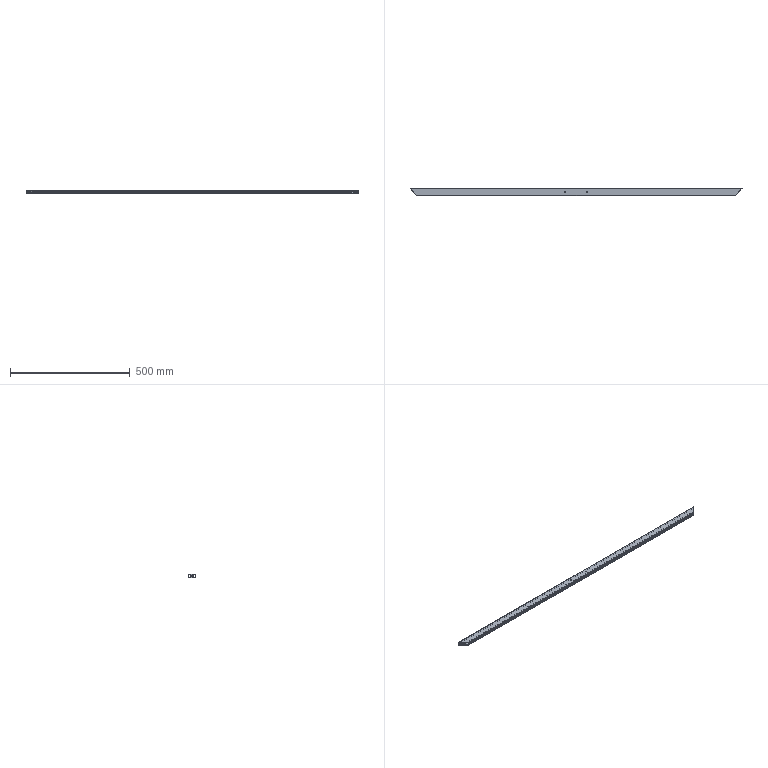Part | SolidWorks | features 3DProfileFeature 1, HoleWzd 1, ICE 1, WeldMemberFeat 1, WeldmentFeature 1 | 1 solid | 40 faces | box 1386 x 30 x 15 mm | volume 334202 mm3 | cylinder 20 | plane 20 | commonest cylinder face diameters 5 x14 3 x4 12 x2
STEP:
#1=CARTESIAN_POINT('',(-45.,-2.5,0.));
#2=VERTEX_POINT('',#1);
#3=CARTESIAN_POINT('',(-47.5,0.,2.5));
#4=VERTEX_POINT('',#3);
#5=CARTESIAN_POINT('',(-45.,-2.5,0.));
#6=CARTESIAN_POINT('',(-46.464,-2.5,1.464));
#7=CARTESIAN_POINT('',(-47.5,-1.464,2.5));
#8=CARTESIAN_POINT('',(-47.5,0.,2.5));
#9=(BOUNDED_CURVE()B_SPLINE_CURVE(3,(#5,#6,#7,#8),.UNSPECIFIED.,.F.,.F.)B_SPLINE_CURVE_WITH_KNOTS((4,4),(4.712,6.283),.UNSPECIFIED.)CURVE()GEOMETRIC_REPRESENTATION_ITEM()RATIONAL_B_SPLINE_CURVE((1.,0.8047,0.8047,1.))REPRESENTATION_ITEM(''));
#10=EDGE_CURVE('',#2,#4,#9,.T.);
#11=ORIENTED_EDGE('',*,*,#10,.T.);
#12=CARTESIAN_POINT('',(-47.5,0.,7.5));
#13=VERTEX_POINT('',#12);
#14=CARTESIAN_POINT('',(-47.5,0.,7.5));
#15=DIRECTION('',(0.,0.,1.));
#16=VECTOR('',#15,1000.);
#17=LINE('',#14,#16);
#18=EDGE_CURVE('',#4,#13,#17,.T.);
#19=ORIENTED_EDGE('',*,*,#18,.T.);
#20=CARTESIAN_POINT('',(-42.5,0.,7.5));
#21=VERTEX_POINT('',#20);
#22=CARTESIAN_POINT('',(-45.,0.,7.5));
#23=DIRECTION('',(0.,0.,1.));
#24=DIRECTION('',(1.,0.,0.));
#25=AXIS2_PLACEMENT_3D('',#22,#23,#24);
#26=CIRCLE('',#25,2.5);
#27=EDGE_CURVE('',#13,#21,#26,.T.);
#28=ORIENTED_EDGE('',*,*,#27,.T.);
#29=CARTESIAN_POINT('',(-42.5,0.,2.5));
#30=VERTEX_POINT('',#29);
#31=CARTESIAN_POINT('',(-42.5,0.,7.5));
#32=DIRECTION('',(0.,0.,1.));
#33=VECTOR('',#32,1000.);
#34=LINE('',#31,#33);
#35=EDGE_CURVE('',#30,#21,#34,.T.);
#36=ORIENTED_EDGE('',*,*,#35,.F.);
#37=CARTESIAN_POINT('',(-42.5,0.,2.5));
#38=CARTESIAN_POINT('',(-42.5,-1.464,2.5));
#39=CARTESIAN_POINT('',(-43.536,-2.5,1.464));
#40=CARTESIAN_POINT('',(-45.,-2.5,0.));
#41=(BOUNDED_CURVE()B_SPLINE_CURVE(3,(#37,#38,#39,#40),.UNSPECIFIED.,.F.,.F.)B_SPLINE_CURVE_WITH_KNOTS((4,4),(3.142,4.712),.UNSPECIFIED.)CURVE()GEOMETRIC_REPRESENTATION_ITEM()RATIONAL_B_SPLINE_CURVE((1.,0.8047,0.8047,1.))REPRESENTATION_ITEM(''));
#42=EDGE_CURVE('',#30,#2,#41,.T.);
#43=ORIENTED_EDGE('',*,*,#42,.T.);
#44=EDGE_LOOP('',(#11,#19,#28,#36,#43));
#45=FACE_OUTER_BOUND('',#44,.T.);
#46=CARTESIAN_POINT('',(-45.,0.,7.5));
#47=DIRECTION('',(0.,0.,1.));
#48=DIRECTION('',(1.,0.,0.));
#49=AXIS2_PLACEMENT_3D('',#46,#47,#48);
#50=CYLINDRICAL_SURFACE('',#49,2.5);
#51=ADVANCED_FACE('',(#45),#50,.F.);
#52=CARTESIAN_POINT('',(-47.5,0.,-7.5));
#53=VERTEX_POINT('',#52);
#54=CARTESIAN_POINT('',(-42.5,0.,-7.5));
#55=VERTEX_POINT('',#54);
#56=CARTESIAN_POINT('',(-45.,0.,-7.5));
#57=DIRECTION('',(0.,0.,1.));
#58=DIRECTION('',(1.,0.,0.));
#59=AXIS2_PLACEMENT_3D('',#56,#57,#58);
#60=CIRCLE('',#59,2.5);
#61=EDGE_CURVE('',#53,#55,#60,.T.);
#62=ORIENTED_EDGE('',*,*,#61,.F.);
#63=CARTESIAN_POINT('',(-47.5,0.,-2.5));
#64=VERTEX_POINT('',#63);
#65=CARTESIAN_POINT('',(-47.5,0.,7.5));
#66=DIRECTION('',(0.,0.,1.));
#67=VECTOR('',#66,1000.);
#68=LINE('',#65,#67);
#69=EDGE_CURVE('',#53,#64,#68,.T.);
#70=ORIENTED_EDGE('',*,*,#69,.T.);
#71=CARTESIAN_POINT('',(-47.5,0.,-2.5));
#72=CARTESIAN_POINT('',(-47.5,-1.464,-2.5));
#73=CARTESIAN_POINT('',(-46.464,-2.5,-1.464));
#74=CARTESIAN_POINT('',(-45.,-2.5,0.));
#75=(BOUNDED_CURVE()B_SPLINE_CURVE(3,(#71,#72,#73,#74),.UNSPECIFIED.,.F.,.F.)B_SPLINE_CURVE_WITH_KNOTS((4,4),(0.,1.571),.UNSPECIFIED.)CURVE()GEOMETRIC_REPRESENTATION_ITEM()RATIONAL_B_SPLINE_CURVE((1.,0.8047,0.8047,1.))REPRESENTATION_ITEM(''));
#76=EDGE_CURVE('',#64,#2,#75,.T.);
#77=ORIENTED_EDGE('',*,*,#76,.T.);
#78=CARTESIAN_POINT('',(-42.5,0.,-2.5));
#79=VERTEX_POINT('',#78);
#80=CARTESIAN_POINT('',(-45.,-2.5,0.));
#81=CARTESIAN_POINT('',(-43.536,-2.5,-1.464));
#82=CARTESIAN_POINT('',(-42.5,-1.464,-2.5));
#83=CARTESIAN_POINT('',(-42.5,0.,-2.5));
#84=(BOUNDED_CURVE()B_SPLINE_CURVE(3,(#80,#81,#82,#83),.UNSPECIFIED.,.F.,.T.)B_SPLINE_CURVE_WITH_KNOTS((4,4),(1.571,3.142),.UNSPECIFIED.)CURVE()GEOMETRIC_REPRESENTATION_ITEM()RATIONAL_B_SPLINE_CURVE((1.,0.8047,0.8047,1.))REPRESENTATION_ITEM(''));
#85=EDGE_CURVE('',#2,#79,#84,.T.);
#86=ORIENTED_EDGE('',*,*,#85,.T.);
#87=CARTESIAN_POINT('',(-42.5,0.,7.5));
#88=DIRECTION('',(0.,0.,1.));
#89=VECTOR('',#88,1000.);
#90=LINE('',#87,#89);
#91=EDGE_CURVE('',#55,#79,#90,.T.);
#92=ORIENTED_EDGE('',*,*,#91,.F.);
#93=EDGE_LOOP('',(#62,#70,#77,#86,#92));
#94=FACE_OUTER_BOUND('',#93,.T.);
#95=CARTESIAN_POINT('',(-45.,0.,7.5));
#96=DIRECTION('',(0.,0.,1.));
#97=DIRECTION('',(1.,0.,0.));
#98=AXIS2_PLACEMENT_3D('',#95,#96,#97);
#99=CYLINDRICAL_SURFACE('',#98,2.5);
#100=ADVANCED_FACE('',(#94),#99,.F.);
#101=CARTESIAN_POINT('',(45.,-2.5,0.));
#102=VERTEX_POINT('',#101);
#103=CARTESIAN_POINT('',(42.5,0.,2.5));
#104=VERTEX_POINT('',#103);
#105=CARTESIAN_POINT('',(45.,-2.5,0.));
#106=CARTESIAN_POINT('',(43.536,-2.5,1.464));
#107=CARTESIAN_POINT('',(42.5,-1.464,2.5));
#108=CARTESIAN_POINT('',(42.5,0.,2.5));
#109=(BOUNDED_CURVE()B_SPLINE_CURVE(3,(#105,#106,#107,#108),.UNSPECIFIED.,.F.,.F.)B_SPLINE_CURVE_WITH_KNOTS((4,4),(4.712,6.283),.UNSPECIFIED.)CURVE()GEOMETRIC_REPRESENTATION_ITEM()RATIONAL_B_SPLINE_CURVE((1.,0.8047,0.8047,1.))REPRESENTATION_ITEM(''));
#110=EDGE_CURVE('',#102,#104,#109,.T.);
#111=ORIENTED_EDGE('',*,*,#110,.T.);
#112=CARTESIAN_POINT('',(42.5,0.,7.5));
#113=VERTEX_POINT('',#112);
#114=CARTESIAN_POINT('',(42.5,0.,7.5));
#115=DIRECTION('',(0.,0.,1.));
#116=VECTOR('',#115,1000.);
#117=LINE('',#114,#116);
#118=EDGE_CURVE('',#104,#113,#117,.T.);
#119=ORIENTED_EDGE('',*,*,#118,.T.);
#120=CARTESIAN_POINT('',(47.5,0.,7.5));
#121=VERTEX_POINT('',#120);
#122=CARTESIAN_POINT('',(45.,0.,7.5));
#123=DIRECTION('',(0.,0.,1.));
#124=DIRECTION('',(1.,0.,0.));
#125=AXIS2_PLACEMENT_3D('',#122,#123,#124);
#126=CIRCLE('',#125,2.5);
#127=EDGE_CURVE('',#113,#121,#126,.T.);
#128=ORIENTED_EDGE('',*,*,#127,.T.);
#129=CARTESIAN_POINT('',(47.5,0.,2.5));
#130=VERTEX_POINT('',#129);
#131=CARTESIAN_POINT('',(47.5,0.,7.5));
#132=DIRECTION('',(0.,0.,1.));
#133=VECTOR('',#132,1000.);
#134=LINE('',#131,#133);
#135=EDGE_CURVE('',#130,#121,#134,.T.);
#136=ORIENTED_EDGE('',*,*,#135,.F.);
#137=CARTESIAN_POINT('',(47.5,0.,2.5));
#138=CARTESIAN_POINT('',(47.5,-1.464,2.5));
#139=CARTESIAN_POINT('',(46.464,-2.5,1.464));
#140=CARTESIAN_POINT('',(45.,-2.5,0.));
#141=(BOUNDED_CURVE()B_SPLINE_CURVE(3,(#137,#138,#139,#140),.UNSPECIFIED.,.F.,.F.)B_SPLINE_CURVE_WITH_KNOTS((4,4),(3.142,4.712),.UNSPECIFIED.)CURVE()GEOMETRIC_REPRESENTATION_ITEM()RATIONAL_B_SPLINE_CURVE((1.,0.8047,0.8047,1.))REPRESENTATION_ITEM(''));
#142=EDGE_CURVE('',#130,#102,#141,.T.);
#143=ORIENTED_EDGE('',*,*,#142,.T.);
#144=EDGE_LOOP('',(#111,#119,#128,#136,#143));
#145=FACE_OUTER_BOUND('',#144,.T.);
#146=CARTESIAN_POINT('',(45.,0.,7.5));
#147=DIRECTION('',(0.,0.,1.));
#148=DIRECTION('',(1.,0.,0.));
#149=AXIS2_PLACEMENT_3D('',#146,#147,#148);
#150=CYLINDRICAL_SURFACE('',#149,2.5);
#151=ADVANCED_FACE('',(#145),#150,.F.);
#152=CARTESIAN_POINT('',(42.5,0.,-7.5));
#153=VERTEX_POINT('',#152);
#154=CARTESIAN_POINT('',(47.5,0.,-7.5));
#155=VERTEX_POINT('',#154);
#156=CARTESIAN_POINT('',(45.,0.,-7.5));
#157=DIRECTION('',(0.,0.,1.));
#158=DIRECTION('',(1.,0.,0.));
#159=AXIS2_PLACEMENT_3D('',#156,#157,#158);
#160=CIRCLE('',#159,2.5);
#161=EDGE_CURVE('',#153,#155,#160,.T.);
#162=ORIENTED_EDGE('',*,*,#161,.F.);
#163=CARTESIAN_POINT('',(42.5,0.,-2.5));
#164=VERTEX_POINT('',#163);
#165=CARTESIAN_POINT('',(42.5,0.,7.5));
#166=DIRECTION('',(0.,0.,1.));
#167=VECTOR('',#166,1000.);
#168=LINE('',#165,#167);
#169=EDGE_CURVE('',#153,#164,#168,.T.);
#170=ORIENTED_EDGE('',*,*,#169,.T.);
#171=CARTESIAN_POINT('',(42.5,0.,-2.5));
#172=CARTESIAN_POINT('',(42.5,-1.464,-2.5));
#173=CARTESIAN_POINT('',(43.536,-2.5,-1.464));
#174=CARTESIAN_POINT('',(45.,-2.5,0.));
#175=(BOUNDED_CURVE()B_SPLINE_CURVE(3,(#171,#172,#173,#174),.UNSPECIFIED.,.F.,.T.)B_SPLINE_CURVE_WITH_KNOTS((4,4),(0.,1.571),.UNSPECIFIED.)CURVE()GEOMETRIC_REPRESENTATION_ITEM()RATIONAL_B_SPLINE_CURVE((1.,0.8047,0.8047,1.))REPRESENTATION_ITEM(''));
#176=EDGE_CURVE('',#164,#102,#175,.T.);
#177=ORIENTED_EDGE('',*,*,#176,.T.);
#178=CARTESIAN_POINT('',(47.5,0.,-2.5));
#179=VERTEX_POINT('',#178);
#180=CARTESIAN_POINT('',(45.,-2.5,0.));
#181=CARTESIAN_POINT('',(46.464,-2.5,-1.464));
#182=CARTESIAN_POINT('',(47.5,-1.464,-2.5));
#183=CARTESIAN_POINT('',(47.5,0.,-2.5));
#184=(BOUNDED_CURVE()B_SPLINE_CURVE(3,(#180,#181,#182,#183),.UNSPECIFIED.,.F.,.F.)B_SPLINE_CURVE_WITH_KNOTS((4,4),(1.571,3.142),.UNSPECIFIED.)CURVE()GEOMETRIC_REPRESENTATION_ITEM()RATIONAL_B_SPLINE_CURVE((1.,0.8047,0.8047,1.))REPRESENTATION_ITEM(''));
#185=EDGE_CURVE('',#102,#179,#184,.T.);
#186=ORIENTED_EDGE('',*,*,#185,.T.);
#187=CARTESIAN_POINT('',(47.5,0.,7.5));
#188=DIRECTION('',(0.,0.,1.));
#189=VECTOR('',#188,1000.);
#190=LINE('',#187,#189);
#191=EDGE_CURVE('',#155,#179,#190,.T.);
#192=ORIENTED_EDGE('',*,*,#191,.F.);
#193=EDGE_LOOP('',(#162,#170,#177,#186,#192));
#194=FACE_OUTER_BOUND('',#193,.T.);
#195=CARTESIAN_POINT('',(45.,0.,7.5));
#196=DIRECTION('',(0.,0.,1.));
#197=DIRECTION('',(1.,0.,0.));
#198=AXIS2_PLACEMENT_3D('',#195,#196,#197);
#199=CYLINDRICAL_SURFACE('',#198,2.5);
#200=ADVANCED_FACE('',(#194),#199,.F.);
#201=ORIENTED_EDGE('',*,*,#76,.F.);
#202=CARTESIAN_POINT('',(-678.,0.,-2.5));
#203=VERTEX_POINT('',#202);
#204=CARTESIAN_POINT('',(693.,0.,-2.5));
#205=DIRECTION('',(-1.,0.,0.));
#206=VECTOR('',#205,1000.);
#207=LINE('',#204,#206);
#208=EDGE_CURVE('',#64,#203,#207,.T.);
#209=ORIENTED_EDGE('',*,*,#208,.T.);
#210=CARTESIAN_POINT('',(-678.,0.,2.5));
#211=VERTEX_POINT('',#210);
#212=CARTESIAN_POINT('',(-678.,0.,2.5));
#213=CARTESIAN_POINT('',(-673.,-5.,2.5));
#214=CARTESIAN_POINT('',(-673.,-5.,-2.5));
#215=CARTESIAN_POINT('',(-678.,0.,-2.5));
#216=(BOUNDED_CURVE()B_SPLINE_CURVE(3,(#212,#213,#214,#215),.UNSPECIFIED.,.F.,.F.)B_SPLINE_CURVE_WITH_KNOTS((4,4),(1.571,4.712),.UNSPECIFIED.)CURVE()GEOMETRIC_REPRESENTATION_ITEM()RATIONAL_B_SPLINE_CURVE((1.,0.3333,0.3333,1.))REPRESENTATION_ITEM(''));
#217=EDGE_CURVE('',#211,#203,#216,.T.);
#218=ORIENTED_EDGE('',*,*,#217,.F.);
#219=CARTESIAN_POINT('',(693.,0.,2.5));
#220=DIRECTION('',(-1.,0.,0.));
#221=VECTOR('',#220,1000.);
#222=LINE('',#219,#221);
#223=EDGE_CURVE('',#4,#211,#222,.T.);
#224=ORIENTED_EDGE('',*,*,#223,.F.);
#225=ORIENTED_EDGE('',*,*,#10,.F.);
#226=EDGE_LOOP('',(#201,#209,#218,#224,#225));
#227=FACE_OUTER_BOUND('',#226,.T.);
#228=CARTESIAN_POINT('',(693.,0.,0.));
#229=DIRECTION('',(-1.,0.,0.));
#230=DIRECTION('',(0.,0.,1.));
#231=AXIS2_PLACEMENT_3D('',#228,#229,#230);
#232=CYLINDRICAL_SURFACE('',#231,2.5);
#233=ADVANCED_FACE('',(#227),#232,.F.);
#234=CARTESIAN_POINT('',(678.,0.,-2.5));
#235=VERTEX_POINT('',#234);
#236=CARTESIAN_POINT('',(678.,0.,2.5));
#237=VERTEX_POINT('',#236);
#238=CARTESIAN_POINT('',(678.,0.,-2.5));
#239=CARTESIAN_POINT('',(673.,-5.,-2.5));
#240=CARTESIAN_POINT('',(673.,-5.,2.5));
#241=CARTESIAN_POINT('',(678.,0.,2.5));
#242=(BOUNDED_CURVE()B_SPLINE_CURVE(3,(#238,#239,#240,#241),.UNSPECIFIED.,.F.,.F.)B_SPLINE_CURVE_WITH_KNOTS((4,4),(4.712,7.854),.UNSPECIFIED.)CURVE()GEOMETRIC_REPRESENTATION_ITEM()RATIONAL_B_SPLINE_CURVE((1.,0.3333,0.3333,1.))REPRESENTATION_ITEM(''));
#243=EDGE_CURVE('',#235,#237,#242,.T.);
#244=ORIENTED_EDGE('',*,*,#243,.F.);
#245=CARTESIAN_POINT('',(693.,0.,-2.5));
#246=DIRECTION('',(-1.,0.,0.));
#247=VECTOR('',#246,1000.);
#248=LINE('',#245,#247);
#249=EDGE_CURVE('',#235,#179,#248,.T.);
#250=ORIENTED_EDGE('',*,*,#249,.T.);
#251=ORIENTED_EDGE('',*,*,#185,.F.);
#252=ORIENTED_EDGE('',*,*,#142,.F.);
#253=CARTESIAN_POINT('',(693.,0.,2.5));
#254=DIRECTION('',(-1.,0.,0.));
#255=VECTOR('',#254,1000.);
#256=LINE('',#253,#255);
#257=EDGE_CURVE('',#237,#130,#256,.T.);
#258=ORIENTED_EDGE('',*,*,#257,.F.);
#259=EDGE_LOOP('',(#244,#250,#251,#252,#258));
#260=FACE_OUTER_BOUND('',#259,.T.);
#261=CARTESIAN_POINT('',(693.,0.,0.));
#262=DIRECTION('',(-1.,0.,0.));
#263=DIRECTION('',(0.,0.,1.));
#264=AXIS2_PLACEMENT_3D('',#261,#262,#263);
#265=CYLINDRICAL_SURFACE('',#264,2.5);
#266=ADVANCED_FACE('',(#260),#265,.F.);
#267=ORIENTED_EDGE('',*,*,#176,.F.);
#268=CARTESIAN_POINT('',(693.,0.,-2.5));
#269=DIRECTION('',(-1.,0.,0.));
#270=VECTOR('',#269,1000.);
#271=LINE('',#268,#270);
#272=EDGE_CURVE('',#164,#79,#271,.T.);
#273=ORIENTED_EDGE('',*,*,#272,.T.);
#274=ORIENTED_EDGE('',*,*,#85,.F.);
#275=ORIENTED_EDGE('',*,*,#42,.F.);
#276=CARTESIAN_POINT('',(693.,0.,2.5));
#277=DIRECTION('',(-1.,0.,0.));
#278=VECTOR('',#277,1000.);
#279=LINE('',#276,#278);
#280=EDGE_CURVE('',#104,#30,#279,.T.);
#281=ORIENTED_EDGE('',*,*,#280,.F.);
#282=ORIENTED_EDGE('',*,*,#110,.F.);
#283=EDGE_LOOP('',(#267,#273,#274,#275,#281,#282));
#284=FACE_OUTER_BOUND('',#283,.T.);
#285=CARTESIAN_POINT('',(693.,0.,0.));
#286=DIRECTION('',(-1.,0.,0.));
#287=DIRECTION('',(0.,0.,1.));
#288=AXIS2_PLACEMENT_3D('',#285,#286,#287);
#289=CYLINDRICAL_SURFACE('',#288,2.5);
#290=ADVANCED_FACE('',(#284),#289,.F.);
#291=ORIENTED_EDGE('',*,*,#272,.F.);
#292=CARTESIAN_POINT('',(45.,2.5,0.));
#293=VERTEX_POINT('',#292);
#294=CARTESIAN_POINT('',(45.,2.5,0.));
#295=CARTESIAN_POINT('',(43.536,2.5,-1.464));
#296=CARTESIAN_POINT('',(42.5,1.464,-2.5));
#297=CARTESIAN_POINT('',(42.5,0.,-2.5));
#298=(BOUNDED_CURVE()B_SPLINE_CURVE(3,(#294,#295,#296,#297),.UNSPECIFIED.,.F.,.F.)B_SPLINE_CURVE_WITH_KNOTS((4,4),(4.712,6.283),.UNSPECIFIED.)CURVE()GEOMETRIC_REPRESENTATION_ITEM()RATIONAL_B_SPLINE_CURVE((1.,0.8047,0.8047,1.))REPRESENTATION_ITEM(''));
#299=EDGE_CURVE('',#293,#164,#298,.T.);
#300=ORIENTED_EDGE('',*,*,#299,.F.);
#301=CARTESIAN_POINT('',(42.5,0.,2.5));
#302=CARTESIAN_POINT('',(42.5,1.464,2.5));
#303=CARTESIAN_POINT('',(43.536,2.5,1.464));
#304=CARTESIAN_POINT('',(45.,2.5,0.));
#305=(BOUNDED_CURVE()B_SPLINE_CURVE(3,(#301,#302,#303,#304),.UNSPECIFIED.,.F.,.F.)B_SPLINE_CURVE_WITH_KNOTS((4,4),(0.,1.571),.UNSPECIFIED.)CURVE()GEOMETRIC_REPRESENTATION_ITEM()RATIONAL_B_SPLINE_CURVE((1.,0.8047,0.8047,1.))REPRESENTATION_ITEM(''));
#306=EDGE_CURVE('',#104,#293,#305,.T.);
#307=ORIENTED_EDGE('',*,*,#306,.F.);
#308=ORIENTED_EDGE('',*,*,#280,.T.);
#309=CARTESIAN_POINT('',(-45.,2.5,0.));
#310=VERTEX_POINT('',#309);
#311=CARTESIAN_POINT('',(-45.,2.5,0.));
#312=CARTESIAN_POINT('',(-43.536,2.5,1.464));
#313=CARTESIAN_POINT('',(-42.5,1.464,2.5));
#314=CARTESIAN_POINT('',(-42.5,0.,2.5));
#315=(BOUNDED_CURVE()B_SPLINE_CURVE(3,(#311,#312,#313,#314),.UNSPECIFIED.,.F.,.F.)B_SPLINE_CURVE_WITH_KNOTS((4,4),(1.571,3.142),.UNSPECIFIED.)CURVE()GEOMETRIC_REPRESENTATION_ITEM()RATIONAL_B_SPLINE_CURVE((1.,0.8047,0.8047,1.))REPRESENTATION_ITEM(''));
#316=EDGE_CURVE('',#310,#30,#315,.T.);
#317=ORIENTED_EDGE('',*,*,#316,.F.);
#318=CARTESIAN_POINT('',(-42.5,0.,-2.5));
#319=CARTESIAN_POINT('',(-42.5,1.464,-2.5));
#320=CARTESIAN_POINT('',(-43.536,2.5,-1.464));
#321=CARTESIAN_POINT('',(-45.,2.5,0.));
#322=(BOUNDED_CURVE()B_SPLINE_CURVE(3,(#318,#319,#320,#321),.UNSPECIFIED.,.F.,.F.)B_SPLINE_CURVE_WITH_KNOTS((4,4),(3.142,4.712),.UNSPECIFIED.)CURVE()GEOMETRIC_REPRESENTATION_ITEM()RATIONAL_B_SPLINE_CURVE((1.,0.8047,0.8047,1.))REPRESENTATION_ITEM(''));
#323=EDGE_CURVE('',#79,#310,#322,.T.);
#324=ORIENTED_EDGE('',*,*,#323,.F.);
#325=EDGE_LOOP('',(#291,#300,#307,#308,#317,#324));
#326=FACE_OUTER_BOUND('',#325,.T.);
#327=CARTESIAN_POINT('',(693.,0.,0.));
#328=DIRECTION('',(-1.,0.,0.));
#329=DIRECTION('',(0.,0.,1.));
#330=AXIS2_PLACEMENT_3D('',#327,#328,#329);
#331=CYLINDRICAL_SURFACE('',#330,2.5);
#332=ADVANCED_FACE('',(#326),#331,.F.);
#333=ORIENTED_EDGE('',*,*,#249,.F.);
#334=CARTESIAN_POINT('',(678.,0.,2.5));
#335=CARTESIAN_POINT('',(683.,5.,2.5));
#336=CARTESIAN_POINT('',(683.,5.,-2.5));
#337=CARTESIAN_POINT('',(678.,0.,-2.5));
#338=(BOUNDED_CURVE()B_SPLINE_CURVE(3,(#334,#335,#336,#337),.UNSPECIFIED.,.F.,.T.)B_SPLINE_CURVE_WITH_KNOTS((4,4),(1.571,4.712),.UNSPECIFIED.)CURVE()GEOMETRIC_REPRESENTATION_ITEM()RATIONAL_B_SPLINE_CURVE((1.,0.3333,0.3333,1.))REPRESENTATION_ITEM(''));
#339=EDGE_CURVE('',#237,#235,#338,.T.);
#340=ORIENTED_EDGE('',*,*,#339,.F.);
#341=ORIENTED_EDGE('',*,*,#257,.T.);
#342=CARTESIAN_POINT('',(45.,2.5,0.));
#343=CARTESIAN_POINT('',(46.464,2.5,1.464));
#344=CARTESIAN_POINT('',(47.5,1.464,2.5));
#345=CARTESIAN_POINT('',(47.5,0.,2.5));
#346=(BOUNDED_CURVE()B_SPLINE_CURVE(3,(#342,#343,#344,#345),.UNSPECIFIED.,.F.,.F.)B_SPLINE_CURVE_WITH_KNOTS((4,4),(1.571,3.142),.UNSPECIFIED.)CURVE()GEOMETRIC_REPRESENTATION_ITEM()RATIONAL_B_SPLINE_CURVE((1.,0.8047,0.8047,1.))REPRESENTATION_ITEM(''));
#347=EDGE_CURVE('',#293,#130,#346,.T.);
#348=ORIENTED_EDGE('',*,*,#347,.F.);
#349=CARTESIAN_POINT('',(47.5,0.,-2.5));
#350=CARTESIAN_POINT('',(47.5,1.464,-2.5));
#351=CARTESIAN_POINT('',(46.464,2.5,-1.464));
#352=CARTESIAN_POINT('',(45.,2.5,0.));
#353=(BOUNDED_CURVE()B_SPLINE_CURVE(3,(#349,#350,#351,#352),.UNSPECIFIED.,.F.,.F.)B_SPLINE_CURVE_WITH_KNOTS((4,4),(3.142,4.712),.UNSPECIFIED.)CURVE()GEOMETRIC_REPRESENTATION_ITEM()RATIONAL_B_SPLINE_CURVE((1.,0.8047,0.8047,1.))REPRESENTATION_ITEM(''));
#354=EDGE_CURVE('',#179,#293,#353,.T.);
#355=ORIENTED_EDGE('',*,*,#354,.F.);
#356=EDGE_LOOP('',(#333,#340,#341,#348,#355));
#357=FACE_OUTER_BOUND('',#356,.T.);
#358=CARTESIAN_POINT('',(693.,0.,0.));
#359=DIRECTION('',(-1.,0.,0.));
#360=DIRECTION('',(0.,0.,1.));
#361=AXIS2_PLACEMENT_3D('',#358,#359,#360);
#362=CYLINDRICAL_SURFACE('',#361,2.5);
#363=ADVANCED_FACE('',(#357),#362,.F.);
#364=CARTESIAN_POINT('',(693.,15.,3.25));
#365=VERTEX_POINT('',#364);
#366=CARTESIAN_POINT('',(-693.,15.,3.25));
#367=VERTEX_POINT('',#366);
#368=CARTESIAN_POINT('',(693.,15.,3.25));
#369=DIRECTION('',(-1.,0.,0.));
#370=VECTOR('',#369,1000.);
#371=LINE('',#368,#370);
#372=EDGE_CURVE('',#365,#367,#371,.T.);
#373=ORIENTED_EDGE('',*,*,#372,.F.);
#374=CARTESIAN_POINT('',(690.7,12.7,3.25));
#375=VERTEX_POINT('',#374);
#376=CARTESIAN_POINT('',(693.,15.,3.25));
#377=DIRECTION('',(-0.7071,-0.7071,0.));
#378=VECTOR('',#377,1000.);
#379=LINE('',#376,#378);
#380=EDGE_CURVE('',#365,#375,#379,.T.);
#381=ORIENTED_EDGE('',*,*,#380,.T.);
#382=CARTESIAN_POINT('',(-690.7,12.7,3.25));
#383=VERTEX_POINT('',#382);
#384=CARTESIAN_POINT('',(693.,12.7,3.25));
#385=DIRECTION('',(-1.,0.,0.));
#386=VECTOR('',#385,1000.);
#387=LINE('',#384,#386);
#388=EDGE_CURVE('',#375,#383,#387,.T.);
#389=ORIENTED_EDGE('',*,*,#388,.T.);
#390=CARTESIAN_POINT('',(0.,-678.,3.25));
#391=DIRECTION('',(-0.7071,0.7071,0.));
#392=VECTOR('',#391,1000.);
#393=LINE('',#390,#392);
#394=EDGE_CURVE('',#383,#367,#393,.T.);
#395=ORIENTED_EDGE('',*,*,#394,.T.);
#396=EDGE_LOOP('',(#373,#381,#389,#395));
#397=FACE_OUTER_BOUND('',#396,.T.);
#398=CARTESIAN_POINT('',(693.,15.,3.25));
#399=DIRECTION('',(0.,0.,1.));
#400=DIRECTION('',(0.,-1.,0.));
#401=AXIS2_PLACEMENT_3D('',#398,#399,#400);
#402=PLANE('',#401);
#403=ADVANCED_FACE('',(#397),#402,.F.);
#404=CARTESIAN_POINT('',(-693.,15.,6.));
#405=VERTEX_POINT('',#404);
#406=CARTESIAN_POINT('',(-693.,15.,6.));
#407=DIRECTION('',(0.,0.,1.));
#408=VECTOR('',#407,1000.);
#409=LINE('',#406,#408);
#410=EDGE_CURVE('',#367,#405,#409,.T.);
#411=ORIENTED_EDGE('',*,*,#410,.T.);
#412=CARTESIAN_POINT('',(693.,15.,6.));
#413=VERTEX_POINT('',#412);
#414=CARTESIAN_POINT('',(693.,15.,6.));
#415=DIRECTION('',(-1.,0.,0.));
#416=VECTOR('',#415,1000.);
#417=LINE('',#414,#416);
#418=EDGE_CURVE('',#413,#405,#417,.T.);
#419=ORIENTED_EDGE('',*,*,#418,.F.);
#420=CARTESIAN_POINT('',(693.,15.,6.));
#421=DIRECTION('',(0.,0.,1.));
#422=VECTOR('',#421,1000.);
#423=LINE('',#420,#422);
#424=EDGE_CURVE('',#365,#413,#423,.T.);
#425=ORIENTED_EDGE('',*,*,#424,.F.);
#426=ORIENTED_EDGE('',*,*,#372,.T.);
#427=EDGE_LOOP('',(#411,#419,#425,#426));
#428=FACE_OUTER_BOUND('',#427,.T.);
#429=CARTESIAN_POINT('',(693.,15.,6.));
#430=DIRECTION('',(0.,-1.,0.));
#431=DIRECTION('',(0.,0.,-1.));
#432=AXIS2_PLACEMENT_3D('',#429,#430,#431);
#433=PLANE('',#432);
#434=ADVANCED_FACE('',(#428),#433,.F.);
#435=CARTESIAN_POINT('',(691.5,13.5,7.5));
#436=VERTEX_POINT('',#435);
#437=CARTESIAN_POINT('',(-691.5,13.5,7.5));
#438=VERTEX_POINT('',#437);
#439=CARTESIAN_POINT('',(693.,13.5,7.5));
#440=DIRECTION('',(-1.,0.,0.));
#441=VECTOR('',#440,1000.);
#442=LINE('',#439,#441);
#443=EDGE_CURVE('',#436,#438,#442,.T.);
#444=ORIENTED_EDGE('',*,*,#443,.F.);
#445=CARTESIAN_POINT('',(691.5,13.5,7.5));
#446=CARTESIAN_POINT('',(692.379,14.379,7.5));
#447=CARTESIAN_POINT('',(693.,15.,6.879));
#448=CARTESIAN_POINT('',(693.,15.,6.));
#449=(BOUNDED_CURVE()B_SPLINE_CURVE(3,(#445,#446,#447,#448),.UNSPECIFIED.,.F.,.F.)B_SPLINE_CURVE_WITH_KNOTS((4,4),(1.571,3.142),.UNSPECIFIED.)CURVE()GEOMETRIC_REPRESENTATION_ITEM()RATIONAL_B_SPLINE_CURVE((1.,0.8047,0.8047,1.))REPRESENTATION_ITEM(''));
#450=EDGE_CURVE('',#436,#413,#449,.T.);
#451=ORIENTED_EDGE('',*,*,#450,.T.);
#452=ORIENTED_EDGE('',*,*,#418,.T.);
#453=CARTESIAN_POINT('',(-693.,15.,6.));
#454=CARTESIAN_POINT('',(-693.,15.,6.879));
#455=CARTESIAN_POINT('',(-692.379,14.379,7.5));
#456=CARTESIAN_POINT('',(-691.5,13.5,7.5));
#457=(BOUNDED_CURVE()B_SPLINE_CURVE(3,(#453,#454,#455,#456),.UNSPECIFIED.,.F.,.F.)B_SPLINE_CURVE_WITH_KNOTS((4,4),(0.,1.571),.UNSPECIFIED.)CURVE()GEOMETRIC_REPRESENTATION_ITEM()RATIONAL_B_SPLINE_CURVE((1.,0.8047,0.8047,1.))REPRESENTATION_ITEM(''));
#458=EDGE_CURVE('',#405,#438,#457,.T.);
#459=ORIENTED_EDGE('',*,*,#458,.T.);
#460=EDGE_LOOP('',(#444,#451,#452,#459));
#461=FACE_OUTER_BOUND('',#460,.T.);
#462=CARTESIAN_POINT('',(693.,13.5,6.));
#463=DIRECTION('',(-1.,0.,0.));
#464=DIRECTION('',(0.,0.,1.));
#465=AXIS2_PLACEMENT_3D('',#462,#463,#464);
#466=CYLINDRICAL_SURFACE('',#465,1.5);
#467=ADVANCED_FACE('',(#461),#466,.T.);
#468=CARTESIAN_POINT('',(-45.,0.,7.5));
#469=DIRECTION('',(0.,0.,1.));
#470=DIRECTION('',(1.,0.,0.));
#471=AXIS2_PLACEMENT_3D('',#468,#469,#470);
#472=CIRCLE('',#471,2.5);
#473=EDGE_CURVE('',#21,#13,#472,.T.);
#474=ORIENTED_EDGE('',*,*,#473,.F.);
#475=ORIENTED_EDGE('',*,*,#27,.F.);
#476=EDGE_LOOP('',(#474,#475));
#477=FACE_BOUND('',#476,.T.);
#478=CARTESIAN_POINT('',(45.,0.,7.5));
#479=DIRECTION('',(0.,0.,1.));
#480=DIRECTION('',(1.,0.,0.));
#481=AXIS2_PLACEMENT_3D('',#478,#479,#480);
#482=CIRCLE('',#481,2.5);
#483=EDGE_CURVE('',#121,#113,#482,.T.);
#484=ORIENTED_EDGE('',*,*,#483,.F.);
#485=ORIENTED_EDGE('',*,*,#127,.F.);
#486=EDGE_LOOP('',(#484,#485));
#487=FACE_BOUND('',#486,.T.);
#488=CARTESIAN_POINT('',(664.5,-13.5,7.5));
#489=VERTEX_POINT('',#488);
#490=CARTESIAN_POINT('',(-664.5,-13.5,7.5));
#491=VERTEX_POINT('',#490);
#492=CARTESIAN_POINT('',(693.,-13.5,7.5));
#493=DIRECTION('',(-1.,0.,0.));
#494=VECTOR('',#493,1000.);
#495=LINE('',#492,#494);
#496=EDGE_CURVE('',#489,#491,#495,.T.);
#497=ORIENTED_EDGE('',*,*,#496,.F.);
#498=CARTESIAN_POINT('',(693.,15.,7.5));
#499=DIRECTION('',(-0.7071,-0.7071,0.));
#500=VECTOR('',#499,1000.);
#501=LINE('',#498,#500);
#502=EDGE_CURVE('',#436,#489,#501,.T.);
#503=ORIENTED_EDGE('',*,*,#502,.F.);
#504=ORIENTED_EDGE('',*,*,#443,.T.);
#505=CARTESIAN_POINT('',(-693.,15.,7.5));
#506=DIRECTION('',(-0.7071,0.7071,0.));
#507=VECTOR('',#506,1000.);
#508=LINE('',#505,#507);
#509=EDGE_CURVE('',#491,#438,#508,.T.);
#510=ORIENTED_EDGE('',*,*,#509,.F.);
#511=EDGE_LOOP('',(#497,#503,#504,#510));
#512=FACE_OUTER_BOUND('',#511,.T.);
#513=CARTESIAN_POINT('',(693.,-13.5,7.5));
#514=DIRECTION('',(0.,0.,-1.));
#515=DIRECTION('',(-1.,0.,0.));
#516=AXIS2_PLACEMENT_3D('',#513,#514,#515);
#517=PLANE('',#516);
#518=ADVANCED_FACE('',(#477,#487,#512),#517,.F.);
#519=CARTESIAN_POINT('',(663.,-15.,6.));
#520=VERTEX_POINT('',#519);
#521=CARTESIAN_POINT('',(-663.,-15.,6.));
#522=VERTEX_POINT('',#521);
#523=CARTESIAN_POINT('',(693.,-15.,6.));
#524=DIRECTION('',(-1.,0.,0.));
#525=VECTOR('',#524,1000.);
#526=LINE('',#523,#525);
#527=EDGE_CURVE('',#520,#522,#526,.T.);
#528=ORIENTED_EDGE('',*,*,#527,.F.);
#529=CARTESIAN_POINT('',(663.,-15.,6.));
#530=CARTESIAN_POINT('',(663.,-15.,6.879));
#531=CARTESIAN_POINT('',(663.621,-14.379,7.5));
#532=CARTESIAN_POINT('',(664.5,-13.5,7.5));
#533=(BOUNDED_CURVE()B_SPLINE_CURVE(3,(#529,#530,#531,#532),.UNSPECIFIED.,.F.,.F.)B_SPLINE_CURVE_WITH_KNOTS((4,4),(0.,1.571),.UNSPECIFIED.)CURVE()GEOMETRIC_REPRESENTATION_ITEM()RATIONAL_B_SPLINE_CURVE((1.,0.8047,0.8047,1.))REPRESENTATION_ITEM(''));
#534=EDGE_CURVE('',#520,#489,#533,.T.);
#535=ORIENTED_EDGE('',*,*,#534,.T.);
#536=ORIENTED_EDGE('',*,*,#496,.T.);
#537=CARTESIAN_POINT('',(-664.5,-13.5,7.5));
#538=CARTESIAN_POINT('',(-663.621,-14.379,7.5));
#539=CARTESIAN_POINT('',(-663.,-15.,6.879));
#540=CARTESIAN_POINT('',(-663.,-15.,6.));
#541=(BOUNDED_CURVE()B_SPLINE_CURVE(3,(#537,#538,#539,#540),.UNSPECIFIED.,.F.,.F.)B_SPLINE_CURVE_WITH_KNOTS((4,4),(1.571,3.142),.UNSPECIFIED.)CURVE()GEOMETRIC_REPRESENTATION_ITEM()RATIONAL_B_SPLINE_CURVE((1.,0.8047,0.8047,1.))REPRESENTATION_ITEM(''));
#542=EDGE_CURVE('',#491,#522,#541,.T.);
#543=ORIENTED_EDGE('',*,*,#542,.T.);
#544=EDGE_LOOP('',(#528,#535,#536,#543));
#545=FACE_OUTER_BOUND('',#544,.T.);
#546=CARTESIAN_POINT('',(693.,-13.5,6.));
#547=DIRECTION('',(-1.,0.,0.));
#548=DIRECTION('',(0.,0.,1.));
#549=AXIS2_PLACEMENT_3D('',#546,#547,#548);
#550=CYLINDRICAL_SURFACE('',#549,1.5);
#551=ADVANCED_FACE('',(#545),#550,.T.);
#552=CARTESIAN_POINT('',(663.,-15.,3.25));
#553=VERTEX_POINT('',#552);
#554=CARTESIAN_POINT('',(-663.,-15.,3.25));
#555=VERTEX_POINT('',#554);
#556=CARTESIAN_POINT('',(693.,-15.,3.25));
#557=DIRECTION('',(-1.,0.,0.));
#558=VECTOR('',#557,1000.);
#559=LINE('',#556,#558);
#560=EDGE_CURVE('',#553,#555,#559,.T.);
#561=ORIENTED_EDGE('',*,*,#560,.F.);
#562=CARTESIAN_POINT('',(663.,-15.,-7.5));
#563=DIRECTION('',(0.,0.,1.));
#564=VECTOR('',#563,1000.);
#565=LINE('',#562,#564);
#566=EDGE_CURVE('',#553,#520,#565,.T.);
#567=ORIENTED_EDGE('',*,*,#566,.T.);
#568=ORIENTED_EDGE('',*,*,#527,.T.);
#569=CARTESIAN_POINT('',(-663.,-15.,-7.5));
#570=DIRECTION('',(0.,0.,1.));
#571=VECTOR('',#570,1000.);
#572=LINE('',#569,#571);
#573=EDGE_CURVE('',#555,#522,#572,.T.);
#574=ORIENTED_EDGE('',*,*,#573,.F.);
#575=EDGE_LOOP('',(#561,#567,#568,#574));
#576=FACE_OUTER_BOUND('',#575,.T.);
#577=CARTESIAN_POINT('',(693.,-15.,6.));
#578=DIRECTION('',(0.,1.,0.));
#579=DIRECTION('',(0.,0.,1.));
#580=AXIS2_PLACEMENT_3D('',#577,#578,#579);
#581=PLANE('',#580);
#582=ADVANCED_FACE('',(#576),#581,.F.);
#583=CARTESIAN_POINT('',(665.3,-12.7,3.25));
#584=VERTEX_POINT('',#583);
#585=CARTESIAN_POINT('',(-665.3,-12.7,3.25));
#586=VERTEX_POINT('',#585);
#587=CARTESIAN_POINT('',(693.,-12.7,3.25));
#588=DIRECTION('',(-1.,0.,0.));
#589=VECTOR('',#588,1000.);
#590=LINE('',#587,#589);
#591=EDGE_CURVE('',#584,#586,#590,.T.);
#592=ORIENTED_EDGE('',*,*,#591,.F.);
#593=CARTESIAN_POINT('',(678.,0.,3.25));
#594=DIRECTION('',(-0.7071,-0.7071,0.));
#595=VECTOR('',#594,1000.);
#596=LINE('',#593,#595);
#597=EDGE_CURVE('',#584,#553,#596,.T.);
#598=ORIENTED_EDGE('',*,*,#597,.T.);
#599=ORIENTED_EDGE('',*,*,#560,.T.);
#600=CARTESIAN_POINT('',(15.,-693.,3.25));
#601=DIRECTION('',(-0.7071,0.7071,0.));
#602=VECTOR('',#601,1000.);
#603=LINE('',#600,#602);
#604=EDGE_CURVE('',#555,#586,#603,.T.);
#605=ORIENTED_EDGE('',*,*,#604,.T.);
#606=EDGE_LOOP('',(#592,#598,#599,#605));
#607=FACE_OUTER_BOUND('',#606,.T.);
#608=CARTESIAN_POINT('',(693.,-15.,3.25));
#609=DIRECTION('',(0.,0.,1.));
#610=DIRECTION('',(0.,-1.,0.));
#611=AXIS2_PLACEMENT_3D('',#608,#609,#610);
#612=PLANE('',#611);
#613=ADVANCED_FACE('',(#607),#612,.F.);
#614=CARTESIAN_POINT('',(665.3,-12.7,5.));
#615=VERTEX_POINT('',#614);
#616=CARTESIAN_POINT('',(-665.3,-12.7,5.));
#617=VERTEX_POINT('',#616);
#618=CARTESIAN_POINT('',(693.,-12.7,5.));
#619=DIRECTION('',(-1.,0.,0.));
#620=VECTOR('',#619,1000.);
#621=LINE('',#618,#620);
#622=EDGE_CURVE('',#615,#617,#621,.T.);
#623=ORIENTED_EDGE('',*,*,#622,.F.);
#624=CARTESIAN_POINT('',(665.3,-12.7,3.25));
#625=DIRECTION('',(0.,0.,-1.));
#626=VECTOR('',#625,1000.);
#627=LINE('',#624,#626);
#628=EDGE_CURVE('',#615,#584,#627,.T.);
#629=ORIENTED_EDGE('',*,*,#628,.T.);
#630=ORIENTED_EDGE('',*,*,#591,.T.);
#631=CARTESIAN_POINT('',(-665.3,-12.7,3.25));
#632=DIRECTION('',(0.,0.,1.));
#633=VECTOR('',#632,1000.);
#634=LINE('',#631,#633);
#635=EDGE_CURVE('',#586,#617,#634,.T.);
#636=ORIENTED_EDGE('',*,*,#635,.T.);
#637=EDGE_LOOP('',(#623,#629,#630,#636));
#638=FACE_OUTER_BOUND('',#637,.T.);
#639=CARTESIAN_POINT('',(693.,-12.7,3.25));
#640=DIRECTION('',(0.,-1.,0.));
#641=DIRECTION('',(0.,0.,-1.));
#642=AXIS2_PLACEMENT_3D('',#639,#640,#641);
#643=PLANE('',#642);
#644=ADVANCED_FACE('',(#638),#643,.F.);
#645=CARTESIAN_POINT('',(671.,-7.,5.));
#646=VERTEX_POINT('',#645);
#647=CARTESIAN_POINT('',(-671.,-7.,5.));
#648=VERTEX_POINT('',#647);
#649=CARTESIAN_POINT('',(693.,-7.,5.));
#650=DIRECTION('',(-1.,0.,0.));
#651=VECTOR('',#650,1000.);
#652=LINE('',#649,#651);
#653=EDGE_CURVE('',#646,#648,#652,.T.);
#654=ORIENTED_EDGE('',*,*,#653,.F.);
#655=CARTESIAN_POINT('',(679.15,1.15,5.));
#656=DIRECTION('',(-0.7071,-0.7071,0.));
#657=VECTOR('',#656,1000.);
#658=LINE('',#655,#657);
#659=EDGE_CURVE('',#646,#615,#658,.T.);
#660=ORIENTED_EDGE('',*,*,#659,.T.);
#661=ORIENTED_EDGE('',*,*,#622,.T.);
#662=CARTESIAN_POINT('',(13.85,-691.85,5.));
#663=DIRECTION('',(-0.7071,0.7071,0.));
#664=VECTOR('',#663,1000.);
#665=LINE('',#662,#664);
#666=EDGE_CURVE('',#617,#648,#665,.T.);
#667=ORIENTED_EDGE('',*,*,#666,.T.);
#668=EDGE_LOOP('',(#654,#660,#661,#667));
#669=FACE_OUTER_BOUND('',#668,.T.);
#670=CARTESIAN_POINT('',(693.,-12.7,5.));
#671=DIRECTION('',(0.,0.,1.));
#672=DIRECTION('',(0.,-1.,0.));
#673=AXIS2_PLACEMENT_3D('',#670,#671,#672);
#674=PLANE('',#673);
#675=ADVANCED_FACE('',(#669),#674,.F.);
#676=CARTESIAN_POINT('',(671.,-7.,-5.));
#677=VERTEX_POINT('',#676);
#678=CARTESIAN_POINT('',(-671.,-7.,-5.));
#679=VERTEX_POINT('',#678);
#680=CARTESIAN_POINT('',(693.,-7.,-5.));
#681=DIRECTION('',(-1.,0.,0.));
#682=VECTOR('',#681,1000.);
#683=LINE('',#680,#682);
#684=EDGE_CURVE('',#677,#679,#683,.T.);
#685=ORIENTED_EDGE('',*,*,#684,.F.);
#686=CARTESIAN_POINT('',(671.,-7.,-5.));
#687=CARTESIAN_POINT('',(674.958,-3.042,-2.375));
#688=CARTESIAN_POINT('',(674.958,-3.042,2.375));
#689=CARTESIAN_POINT('',(671.,-7.,5.));
#690=(BOUNDED_CURVE()B_SPLINE_CURVE(3,(#686,#687,#688,#689),.UNSPECIFIED.,.F.,.F.)B_SPLINE_CURVE_WITH_KNOTS((4,4),(2.156,4.127),.UNSPECIFIED.)CURVE()GEOMETRIC_REPRESENTATION_ITEM()RATIONAL_B_SPLINE_CURVE((1.,0.7018,0.7018,1.))REPRESENTATION_ITEM(''));
#691=EDGE_CURVE('',#677,#646,#690,.T.);
#692=ORIENTED_EDGE('',*,*,#691,.T.);
#693=ORIENTED_EDGE('',*,*,#653,.T.);
#694=CARTESIAN_POINT('',(-671.,-7.,5.));
#695=CARTESIAN_POINT('',(-674.958,-3.042,2.375));
#696=CARTESIAN_POINT('',(-674.958,-3.042,-2.375));
#697=CARTESIAN_POINT('',(-671.,-7.,-5.));
#698=(BOUNDED_CURVE()B_SPLINE_CURVE(3,(#694,#695,#696,#697),.UNSPECIFIED.,.F.,.F.)B_SPLINE_CURVE_WITH_KNOTS((4,4),(5.298,7.268),.UNSPECIFIED.)CURVE()GEOMETRIC_REPRESENTATION_ITEM()RATIONAL_B_SPLINE_CURVE((1.,0.7018,0.7018,1.))REPRESENTATION_ITEM(''));
#699=EDGE_CURVE('',#648,#679,#698,.T.);
#700=ORIENTED_EDGE('',*,*,#699,.T.);
#701=EDGE_LOOP('',(#685,#692,#693,#700));
#702=FACE_OUTER_BOUND('',#701,.T.);
#703=CARTESIAN_POINT('',(693.,-10.317,0.));
#704=DIRECTION('',(-1.,0.,0.));
#705=DIRECTION('',(0.,0.,1.));
#706=AXIS2_PLACEMENT_3D('',#703,#704,#705);
#707=CYLINDRICAL_SURFACE('',#706,6.);
#708=ADVANCED_FACE('',(#702),#707,.F.);
#709=CARTESIAN_POINT('',(665.3,-12.7,-5.));
#710=VERTEX_POINT('',#709);
#711=CARTESIAN_POINT('',(-665.3,-12.7,-5.));
#712=VERTEX_POINT('',#711);
#713=CARTESIAN_POINT('',(693.,-12.7,-5.));
#714=DIRECTION('',(-1.,0.,0.));
#715=VECTOR('',#714,1000.);
#716=LINE('',#713,#715);
#717=EDGE_CURVE('',#710,#712,#716,.T.);
#718=ORIENTED_EDGE('',*,*,#717,.F.);
#719=CARTESIAN_POINT('',(679.15,1.15,-5.));
#720=DIRECTION('',(0.7071,0.7071,0.));
#721=VECTOR('',#720,1000.);
#722=LINE('',#719,#721);
#723=EDGE_CURVE('',#710,#677,#722,.T.);
#724=ORIENTED_EDGE('',*,*,#723,.T.);
#725=ORIENTED_EDGE('',*,*,#684,.T.);
#726=CARTESIAN_POINT('',(13.85,-691.85,-5.));
#727=DIRECTION('',(0.7071,-0.7071,0.));
#728=VECTOR('',#727,1000.);
#729=LINE('',#726,#728);
#730=EDGE_CURVE('',#679,#712,#729,.T.);
#731=ORIENTED_EDGE('',*,*,#730,.T.);
#732=EDGE_LOOP('',(#718,#724,#725,#731));
#733=FACE_OUTER_BOUND('',#732,.T.);
#734=CARTESIAN_POINT('',(693.,-12.7,-5.));
#735=DIRECTION('',(0.,0.,-1.));
#736=DIRECTION('',(0.,1.,0.));
#737=AXIS2_PLACEMENT_3D('',#734,#735,#736);
#738=PLANE('',#737);
#739=ADVANCED_FACE('',(#733),#738,.F.);
#740=CARTESIAN_POINT('',(665.3,-12.7,-3.25));
#741=VERTEX_POINT('',#740);
#742=CARTESIAN_POINT('',(-665.3,-12.7,-3.25));
#743=VERTEX_POINT('',#742);
#744=CARTESIAN_POINT('',(693.,-12.7,-3.25));
#745=DIRECTION('',(-1.,0.,0.));
#746=VECTOR('',#745,1000.);
#747=LINE('',#744,#746);
#748=EDGE_CURVE('',#741,#743,#747,.T.);
#749=ORIENTED_EDGE('',*,*,#748,.F.);
#750=CARTESIAN_POINT('',(665.3,-12.7,-3.25));
#751=DIRECTION('',(0.,0.,-1.));
#752=VECTOR('',#751,1000.);
#753=LINE('',#750,#752);
#754=EDGE_CURVE('',#741,#710,#753,.T.);
#755=ORIENTED_EDGE('',*,*,#754,.T.);
#756=ORIENTED_EDGE('',*,*,#717,.T.);
#757=CARTESIAN_POINT('',(-665.3,-12.7,-3.25));
#758=DIRECTION('',(0.,0.,1.));
#759=VECTOR('',#758,1000.);
#760=LINE('',#757,#759);
#761=EDGE_CURVE('',#712,#743,#760,.T.);
#762=ORIENTED_EDGE('',*,*,#761,.T.);
#763=EDGE_LOOP('',(#749,#755,#756,#762));
#764=FACE_OUTER_BOUND('',#763,.T.);
#765=CARTESIAN_POINT('',(693.,-12.7,-3.25));
#766=DIRECTION('',(0.,-1.,0.));
#767=DIRECTION('',(0.,0.,-1.));
#768=AXIS2_PLACEMENT_3D('',#765,#766,#767);
#769=PLANE('',#768);
#770=ADVANCED_FACE('',(#764),#769,.F.);
#771=CARTESIAN_POINT('',(663.,-15.,-3.25));
#772=VERTEX_POINT('',#771);
#773=CARTESIAN_POINT('',(-663.,-15.,-3.25));
#774=VERTEX_POINT('',#773);
#775=CARTESIAN_POINT('',(693.,-15.,-3.25));
#776=DIRECTION('',(-1.,0.,0.));
#777=VECTOR('',#776,1000.);
#778=LINE('',#775,#777);
#779=EDGE_CURVE('',#772,#774,#778,.T.);
#780=ORIENTED_EDGE('',*,*,#779,.F.);
#781=CARTESIAN_POINT('',(678.,0.,-3.25));
#782=DIRECTION('',(0.7071,0.7071,0.));
#783=VECTOR('',#782,1000.);
#784=LINE('',#781,#783);
#785=EDGE_CURVE('',#772,#741,#784,.T.);
#786=ORIENTED_EDGE('',*,*,#785,.T.);
#787=ORIENTED_EDGE('',*,*,#748,.T.);
#788=CARTESIAN_POINT('',(15.,-693.,-3.25));
#789=DIRECTION('',(0.7071,-0.7071,0.));
#790=VECTOR('',#789,1000.);
#791=LINE('',#788,#790);
#792=EDGE_CURVE('',#743,#774,#791,.T.);
#793=ORIENTED_EDGE('',*,*,#792,.T.);
#794=EDGE_LOOP('',(#780,#786,#787,#793));
#795=FACE_OUTER_BOUND('',#794,.T.);
#796=CARTESIAN_POINT('',(693.,-15.,-3.25));
#797=DIRECTION('',(0.,0.,-1.));
#798=DIRECTION('',(0.,1.,0.));
#799=AXIS2_PLACEMENT_3D('',#796,#797,#798);
#800=PLANE('',#799);
#801=ADVANCED_FACE('',(#795),#800,.F.);
#802=CARTESIAN_POINT('',(663.,-15.,-6.));
#803=VERTEX_POINT('',#802);
#804=CARTESIAN_POINT('',(-663.,-15.,-6.));
#805=VERTEX_POINT('',#804);
#806=CARTESIAN_POINT('',(693.,-15.,-6.));
#807=DIRECTION('',(-1.,0.,0.));
#808=VECTOR('',#807,1000.);
#809=LINE('',#806,#808);
#810=EDGE_CURVE('',#803,#805,#809,.T.);
#811=ORIENTED_EDGE('',*,*,#810,.F.);
#812=CARTESIAN_POINT('',(663.,-15.,-7.5));
#813=DIRECTION('',(0.,0.,1.));
#814=VECTOR('',#813,1000.);
#815=LINE('',#812,#814);
#816=EDGE_CURVE('',#803,#772,#815,.T.);
#817=ORIENTED_EDGE('',*,*,#816,.T.);
#818=ORIENTED_EDGE('',*,*,#779,.T.);
#819=CARTESIAN_POINT('',(-663.,-15.,-7.5));
#820=DIRECTION('',(0.,0.,1.));
#821=VECTOR('',#820,1000.);
#822=LINE('',#819,#821);
#823=EDGE_CURVE('',#805,#774,#822,.T.);
#824=ORIENTED_EDGE('',*,*,#823,.F.);
#825=EDGE_LOOP('',(#811,#817,#818,#824));
#826=FACE_OUTER_BOUND('',#825,.T.);
#827=CARTESIAN_POINT('',(693.,-15.,-3.25));
#828=DIRECTION('',(0.,1.,0.));
#829=DIRECTION('',(0.,0.,1.));
#830=AXIS2_PLACEMENT_3D('',#827,#828,#829);
#831=PLANE('',#830);
#832=ADVANCED_FACE('',(#826),#831,.F.);
#833=CARTESIAN_POINT('',(664.5,-13.5,-7.5));
#834=VERTEX_POINT('',#833);
#835=CARTESIAN_POINT('',(-664.5,-13.5,-7.5));
#836=VERTEX_POINT('',#835);
#837=CARTESIAN_POINT('',(693.,-13.5,-7.5));
#838=DIRECTION('',(-1.,0.,0.));
#839=VECTOR('',#838,1000.);
#840=LINE('',#837,#839);
#841=EDGE_CURVE('',#834,#836,#840,.T.);
#842=ORIENTED_EDGE('',*,*,#841,.F.);
#843=CARTESIAN_POINT('',(664.5,-13.5,-7.5));
#844=CARTESIAN_POINT('',(663.621,-14.379,-7.5));
#845=CARTESIAN_POINT('',(663.,-15.,-6.879));
#846=CARTESIAN_POINT('',(663.,-15.,-6.));
#847=(BOUNDED_CURVE()B_SPLINE_CURVE(3,(#843,#844,#845,#846),.UNSPECIFIED.,.F.,.F.)B_SPLINE_CURVE_WITH_KNOTS((4,4),(4.712,6.283),.UNSPECIFIED.)CURVE()GEOMETRIC_REPRESENTATION_ITEM()RATIONAL_B_SPLINE_CURVE((1.,0.8047,0.8047,1.))REPRESENTATION_ITEM(''));
#848=EDGE_CURVE('',#834,#803,#847,.T.);
#849=ORIENTED_EDGE('',*,*,#848,.T.);
#850=ORIENTED_EDGE('',*,*,#810,.T.);
#851=CARTESIAN_POINT('',(-663.,-15.,-6.));
#852=CARTESIAN_POINT('',(-663.,-15.,-6.879));
#853=CARTESIAN_POINT('',(-663.621,-14.379,-7.5));
#854=CARTESIAN_POINT('',(-664.5,-13.5,-7.5));
#855=(BOUNDED_CURVE()B_SPLINE_CURVE(3,(#851,#852,#853,#854),.UNSPECIFIED.,.F.,.F.)B_SPLINE_CURVE_WITH_KNOTS((4,4),(3.142,4.712),.UNSPECIFIED.)CURVE()GEOMETRIC_REPRESENTATION_ITEM()RATIONAL_B_SPLINE_CURVE((1.,0.8047,0.8047,1.))REPRESENTATION_ITEM(''));
#856=EDGE_CURVE('',#805,#836,#855,.T.);
#857=ORIENTED_EDGE('',*,*,#856,.T.);
#858=EDGE_LOOP('',(#842,#849,#850,#857));
#859=FACE_OUTER_BOUND('',#858,.T.);
#860=CARTESIAN_POINT('',(693.,-13.5,-6.));
#861=DIRECTION('',(-1.,0.,0.));
#862=DIRECTION('',(0.,0.,1.));
#863=AXIS2_PLACEMENT_3D('',#860,#861,#862);
#864=CYLINDRICAL_SURFACE('',#863,1.5);
#865=ADVANCED_FACE('',(#859),#864,.T.);
#866=CARTESIAN_POINT('',(-45.,0.,-7.5));
#867=DIRECTION('',(0.,0.,1.));
#868=DIRECTION('',(1.,0.,0.));
#869=AXIS2_PLACEMENT_3D('',#866,#867,#868);
#870=CIRCLE('',#869,2.5);
#871=EDGE_CURVE('',#55,#53,#870,.T.);
#872=ORIENTED_EDGE('',*,*,#871,.T.);
#873=ORIENTED_EDGE('',*,*,#61,.T.);
#874=EDGE_LOOP('',(#872,#873));
#875=FACE_BOUND('',#874,.T.);
#876=CARTESIAN_POINT('',(45.,0.,-7.5));
#877=DIRECTION('',(0.,0.,1.));
#878=DIRECTION('',(1.,0.,0.));
#879=AXIS2_PLACEMENT_3D('',#876,#877,#878);
#880=CIRCLE('',#879,2.5);
#881=EDGE_CURVE('',#155,#153,#880,.T.);
#882=ORIENTED_EDGE('',*,*,#881,.T.);
#883=ORIENTED_EDGE('',*,*,#161,.T.);
#884=EDGE_LOOP('',(#882,#883));
#885=FACE_BOUND('',#884,.T.);
#886=CARTESIAN_POINT('',(691.5,13.5,-7.5));
#887=VERTEX_POINT('',#886);
#888=CARTESIAN_POINT('',(-691.5,13.5,-7.5));
#889=VERTEX_POINT('',#888);
#890=CARTESIAN_POINT('',(693.,13.5,-7.5));
#891=DIRECTION('',(-1.,0.,0.));
#892=VECTOR('',#891,1000.);
#893=LINE('',#890,#892);
#894=EDGE_CURVE('',#887,#889,#893,.T.);
#895=ORIENTED_EDGE('',*,*,#894,.F.);
#896=CARTESIAN_POINT('',(693.,15.,-7.5));
#897=DIRECTION('',(-0.7071,-0.7071,0.));
#898=VECTOR('',#897,1000.);
#899=LINE('',#896,#898);
#900=EDGE_CURVE('',#887,#834,#899,.T.);
#901=ORIENTED_EDGE('',*,*,#900,.T.);
#902=ORIENTED_EDGE('',*,*,#841,.T.);
#903=CARTESIAN_POINT('',(-693.,15.,-7.5));
#904=DIRECTION('',(-0.7071,0.7071,0.));
#905=VECTOR('',#904,1000.);
#906=LINE('',#903,#905);
#907=EDGE_CURVE('',#836,#889,#906,.T.);
#908=ORIENTED_EDGE('',*,*,#907,.T.);
#909=EDGE_LOOP('',(#895,#901,#902,#908));
#910=FACE_OUTER_BOUND('',#909,.T.);
#911=CARTESIAN_POINT('',(693.,-13.5,-7.5));
#912=DIRECTION('',(0.,0.,1.));
#913=DIRECTION('',(1.,0.,0.));
#914=AXIS2_PLACEMENT_3D('',#911,#912,#913);
#915=PLANE('',#914);
#916=ADVANCED_FACE('',(#875,#885,#910),#915,.F.);
#917=CARTESIAN_POINT('',(693.,15.,-6.));
#918=VERTEX_POINT('',#917);
#919=CARTESIAN_POINT('',(-693.,15.,-6.));
#920=VERTEX_POINT('',#919);
#921=CARTESIAN_POINT('',(693.,15.,-6.));
#922=DIRECTION('',(-1.,0.,0.));
#923=VECTOR('',#922,1000.);
#924=LINE('',#921,#923);
#925=EDGE_CURVE('',#918,#920,#924,.T.);
#926=ORIENTED_EDGE('',*,*,#925,.F.);
#927=CARTESIAN_POINT('',(693.,15.,-6.));
#928=CARTESIAN_POINT('',(693.,15.,-6.879));
#929=CARTESIAN_POINT('',(692.379,14.379,-7.5));
#930=CARTESIAN_POINT('',(691.5,13.5,-7.5));
#931=(BOUNDED_CURVE()B_SPLINE_CURVE(3,(#927,#928,#929,#930),.UNSPECIFIED.,.F.,.F.)B_SPLINE_CURVE_WITH_KNOTS((4,4),(3.142,4.712),.UNSPECIFIED.)CURVE()GEOMETRIC_REPRESENTATION_ITEM()RATIONAL_B_SPLINE_CURVE((1.,0.8047,0.8047,1.))REPRESENTATION_ITEM(''));
#932=EDGE_CURVE('',#918,#887,#931,.T.);
#933=ORIENTED_EDGE('',*,*,#932,.T.);
#934=ORIENTED_EDGE('',*,*,#894,.T.);
#935=CARTESIAN_POINT('',(-691.5,13.5,-7.5));
#936=CARTESIAN_POINT('',(-692.379,14.379,-7.5));
#937=CARTESIAN_POINT('',(-693.,15.,-6.879));
#938=CARTESIAN_POINT('',(-693.,15.,-6.));
#939=(BOUNDED_CURVE()B_SPLINE_CURVE(3,(#935,#936,#937,#938),.UNSPECIFIED.,.F.,.F.)B_SPLINE_CURVE_WITH_KNOTS((4,4),(4.712,6.283),.UNSPECIFIED.)CURVE()GEOMETRIC_REPRESENTATION_ITEM()RATIONAL_B_SPLINE_CURVE((1.,0.8047,0.8047,1.))REPRESENTATION_ITEM(''));
#940=EDGE_CURVE('',#889,#920,#939,.T.);
#941=ORIENTED_EDGE('',*,*,#940,.T.);
#942=EDGE_LOOP('',(#926,#933,#934,#941));
#943=FACE_OUTER_BOUND('',#942,.T.);
#944=CARTESIAN_POINT('',(693.,13.5,-6.));
#945=DIRECTION('',(-1.,0.,0.));
#946=DIRECTION('',(0.,0.,1.));
#947=AXIS2_PLACEMENT_3D('',#944,#945,#946);
#948=CYLINDRICAL_SURFACE('',#947,1.5);
#949=ADVANCED_FACE('',(#943),#948,.T.);
#950=CARTESIAN_POINT('',(-693.,15.,-3.25));
#951=VERTEX_POINT('',#950);
#952=CARTESIAN_POINT('',(-693.,15.,-3.25));
#953=DIRECTION('',(0.,0.,1.));
#954=VECTOR('',#953,1000.);
#955=LINE('',#952,#954);
#956=EDGE_CURVE('',#920,#951,#955,.T.);
#957=ORIENTED_EDGE('',*,*,#956,.T.);
#958=CARTESIAN_POINT('',(693.,15.,-3.25));
#959=VERTEX_POINT('',#958);
#960=CARTESIAN_POINT('',(693.,15.,-3.25));
#961=DIRECTION('',(-1.,0.,0.));
#962=VECTOR('',#961,1000.);
#963=LINE('',#960,#962);
#964=EDGE_CURVE('',#959,#951,#963,.T.);
#965=ORIENTED_EDGE('',*,*,#964,.F.);
#966=CARTESIAN_POINT('',(693.,15.,-3.25));
#967=DIRECTION('',(0.,0.,1.));
#968=VECTOR('',#967,1000.);
#969=LINE('',#966,#968);
#970=EDGE_CURVE('',#918,#959,#969,.T.);
#971=ORIENTED_EDGE('',*,*,#970,.F.);
#972=ORIENTED_EDGE('',*,*,#925,.T.);
#973=EDGE_LOOP('',(#957,#965,#971,#972));
#974=FACE_OUTER_BOUND('',#973,.T.);
#975=CARTESIAN_POINT('',(693.,15.,-3.25));
#976=DIRECTION('',(0.,-1.,0.));
#977=DIRECTION('',(0.,0.,-1.));
#978=AXIS2_PLACEMENT_3D('',#975,#976,#977);
#979=PLANE('',#978);
#980=ADVANCED_FACE('',(#974),#979,.F.);
#981=CARTESIAN_POINT('',(690.7,12.7,-3.25));
#982=VERTEX_POINT('',#981);
#983=CARTESIAN_POINT('',(-690.7,12.7,-3.25));
#984=VERTEX_POINT('',#983);
#985=CARTESIAN_POINT('',(693.,12.7,-3.25));
#986=DIRECTION('',(-1.,0.,0.));
#987=VECTOR('',#986,1000.);
#988=LINE('',#985,#987);
#989=EDGE_CURVE('',#982,#984,#988,.T.);
#990=ORIENTED_EDGE('',*,*,#989,.F.);
#991=CARTESIAN_POINT('',(693.,15.,-3.25));
#992=DIRECTION('',(0.7071,0.7071,0.));
#993=VECTOR('',#992,1000.);
#994=LINE('',#991,#993);
#995=EDGE_CURVE('',#982,#959,#994,.T.);
#996=ORIENTED_EDGE('',*,*,#995,.T.);
#997=ORIENTED_EDGE('',*,*,#964,.T.);
#998=CARTESIAN_POINT('',(0.,-678.,-3.25));
#999=DIRECTION('',(0.7071,-0.7071,0.));
#1000=VECTOR('',#999,1000.);
#1001=LINE('',#998,#1000);
#1002=EDGE_CURVE('',#951,#984,#1001,.T.);
#1003=ORIENTED_EDGE('',*,*,#1002,.T.);
#1004=EDGE_LOOP('',(#990,#996,#997,#1003));
#1005=FACE_OUTER_BOUND('',#1004,.T.);
#1006=CARTESIAN_POINT('',(693.,15.,-3.25));
#1007=DIRECTION('',(0.,0.,-1.));
#1008=DIRECTION('',(0.,1.,0.));
#1009=AXIS2_PLACEMENT_3D('',#1006,#1007,#1008);
#1010=PLANE('',#1009);
#1011=ADVANCED_FACE('',(#1005),#1010,.F.);
#1012=CARTESIAN_POINT('',(690.7,12.7,-5.));
#1013=VERTEX_POINT('',#1012);
#1014=CARTESIAN_POINT('',(-690.7,12.7,-5.));
#1015=VERTEX_POINT('',#1014);
#1016=CARTESIAN_POINT('',(693.,12.7,-5.));
#1017=DIRECTION('',(-1.,0.,0.));
#1018=VECTOR('',#1017,1000.);
#1019=LINE('',#1016,#1018);
#1020=EDGE_CURVE('',#1013,#1015,#1019,.T.);
#1021=ORIENTED_EDGE('',*,*,#1020,.F.);
#1022=CARTESIAN_POINT('',(690.7,12.7,-3.25));
#1023=DIRECTION('',(0.,0.,1.));
#1024=VECTOR('',#1023,1000.);
#1025=LINE('',#1022,#1024);
#1026=EDGE_CURVE('',#1013,#982,#1025,.T.);
#1027=ORIENTED_EDGE('',*,*,#1026,.T.);
#1028=ORIENTED_EDGE('',*,*,#989,.T.);
#1029=CARTESIAN_POINT('',(-690.7,12.7,-3.25));
#1030=DIRECTION('',(0.,0.,-1.));
#1031=VECTOR('',#1030,1000.);
#1032=LINE('',#1029,#1031);
#1033=EDGE_CURVE('',#984,#1015,#1032,.T.);
#1034=ORIENTED_EDGE('',*,*,#1033,.T.);
#1035=EDGE_LOOP('',(#1021,#1027,#1028,#1034));
#1036=FACE_OUTER_BOUND('',#1035,.T.);
#1037=CARTESIAN_POINT('',(693.,12.7,-3.25));
#1038=DIRECTION('',(0.,1.,0.));
#1039=DIRECTION('',(0.,0.,1.));
#1040=AXIS2_PLACEMENT_3D('',#1037,#1038,#1039);
#1041=PLANE('',#1040);
#1042=ADVANCED_FACE('',(#1036),#1041,.F.);
#1043=CARTESIAN_POINT('',(685.,7.,-5.));
#1044=VERTEX_POINT('',#1043);
#1045=CARTESIAN_POINT('',(-685.,7.,-5.));
#1046=VERTEX_POINT('',#1045);
#1047=CARTESIAN_POINT('',(693.,7.,-5.));
#1048=DIRECTION('',(-1.,0.,0.));
#1049=VECTOR('',#1048,1000.);
#1050=LINE('',#1047,#1049);
#1051=EDGE_CURVE('',#1044,#1046,#1050,.T.);
#1052=ORIENTED_EDGE('',*,*,#1051,.F.);
#1053=CARTESIAN_POINT('',(691.85,13.85,-5.));
#1054=DIRECTION('',(0.7071,0.7071,0.));
#1055=VECTOR('',#1054,1000.);
#1056=LINE('',#1053,#1055);
#1057=EDGE_CURVE('',#1044,#1013,#1056,.T.);
#1058=ORIENTED_EDGE('',*,*,#1057,.T.);
#1059=ORIENTED_EDGE('',*,*,#1020,.T.);
#1060=CARTESIAN_POINT('',(1.15,-679.15,-5.));
#1061=DIRECTION('',(0.7071,-0.7071,0.));
#1062=VECTOR('',#1061,1000.);
#1063=LINE('',#1060,#1062);
#1064=EDGE_CURVE('',#1015,#1046,#1063,.T.);
#1065=ORIENTED_EDGE('',*,*,#1064,.T.);
#1066=EDGE_LOOP('',(#1052,#1058,#1059,#1065));
#1067=FACE_OUTER_BOUND('',#1066,.T.);
#1068=CARTESIAN_POINT('',(693.,12.7,-5.));
#1069=DIRECTION('',(0.,0.,-1.));
#1070=DIRECTION('',(0.,1.,0.));
#1071=AXIS2_PLACEMENT_3D('',#1068,#1069,#1070);
#1072=PLANE('',#1071);
#1073=ADVANCED_FACE('',(#1067),#1072,.F.);
#1074=CARTESIAN_POINT('',(685.,7.,5.));
#1075=VERTEX_POINT('',#1074);
#1076=CARTESIAN_POINT('',(-685.,7.,5.));
#1077=VERTEX_POINT('',#1076);
#1078=CARTESIAN_POINT('',(693.,7.,5.));
#1079=DIRECTION('',(-1.,0.,0.));
#1080=VECTOR('',#1079,1000.);
#1081=LINE('',#1078,#1080);
#1082=EDGE_CURVE('',#1075,#1077,#1081,.T.);
#1083=ORIENTED_EDGE('',*,*,#1082,.F.);
#1084=CARTESIAN_POINT('',(685.,7.,5.));
#1085=CARTESIAN_POINT('',(681.042,3.042,2.375));
#1086=CARTESIAN_POINT('',(681.042,3.042,-2.375));
#1087=CARTESIAN_POINT('',(685.,7.,-5.));
#1088=(BOUNDED_CURVE()B_SPLINE_CURVE(3,(#1084,#1085,#1086,#1087),.UNSPECIFIED.,.F.,.F.)B_SPLINE_CURVE_WITH_KNOTS((4,4),(5.298,7.268),.UNSPECIFIED.)CURVE()GEOMETRIC_REPRESENTATION_ITEM()RATIONAL_B_SPLINE_CURVE((1.,0.7018,0.7018,1.))REPRESENTATION_ITEM(''));
#1089=EDGE_CURVE('',#1075,#1044,#1088,.T.);
#1090=ORIENTED_EDGE('',*,*,#1089,.T.);
#1091=ORIENTED_EDGE('',*,*,#1051,.T.);
#1092=CARTESIAN_POINT('',(-685.,7.,-5.));
#1093=CARTESIAN_POINT('',(-681.042,3.042,-2.375));
#1094=CARTESIAN_POINT('',(-681.042,3.042,2.375));
#1095=CARTESIAN_POINT('',(-685.,7.,5.));
#1096=(BOUNDED_CURVE()B_SPLINE_CURVE(3,(#1092,#1093,#1094,#1095),.UNSPECIFIED.,.F.,.F.)B_SPLINE_CURVE_WITH_KNOTS((4,4),(2.156,4.127),.UNSPECIFIED.)CURVE()GEOMETRIC_REPRESENTATION_ITEM()RATIONAL_B_SPLINE_CURVE((1.,0.7018,0.7018,1.))REPRESENTATION_ITEM(''));
#1097=EDGE_CURVE('',#1046,#1077,#1096,.T.);
#1098=ORIENTED_EDGE('',*,*,#1097,.T.);
#1099=EDGE_LOOP('',(#1083,#1090,#1091,#1098));
#1100=FACE_OUTER_BOUND('',#1099,.T.);
#1101=CARTESIAN_POINT('',(693.,10.317,0.));
#1102=DIRECTION('',(-1.,0.,0.));
#1103=DIRECTION('',(0.,0.,1.));
#1104=AXIS2_PLACEMENT_3D('',#1101,#1102,#1103);
#1105=CYLINDRICAL_SURFACE('',#1104,6.);
#1106=ADVANCED_FACE('',(#1100),#1105,.F.);
#1107=CARTESIAN_POINT('',(690.7,12.7,5.));
#1108=VERTEX_POINT('',#1107);
#1109=CARTESIAN_POINT('',(-690.7,12.7,5.));
#1110=VERTEX_POINT('',#1109);
#1111=CARTESIAN_POINT('',(693.,12.7,5.));
#1112=DIRECTION('',(-1.,0.,0.));
#1113=VECTOR('',#1112,1000.);
#1114=LINE('',#1111,#1113);
#1115=EDGE_CURVE('',#1108,#1110,#1114,.T.);
#1116=ORIENTED_EDGE('',*,*,#1115,.F.);
#1117=CARTESIAN_POINT('',(691.85,13.85,5.));
#1118=DIRECTION('',(-0.7071,-0.7071,0.));
#1119=VECTOR('',#1118,1000.);
#1120=LINE('',#1117,#1119);
#1121=EDGE_CURVE('',#1108,#1075,#1120,.T.);
#1122=ORIENTED_EDGE('',*,*,#1121,.T.);
#1123=ORIENTED_EDGE('',*,*,#1082,.T.);
#1124=CARTESIAN_POINT('',(1.15,-679.15,5.));
#1125=DIRECTION('',(-0.7071,0.7071,0.));
#1126=VECTOR('',#1125,1000.);
#1127=LINE('',#1124,#1126);
#1128=EDGE_CURVE('',#1077,#1110,#1127,.T.);
#1129=ORIENTED_EDGE('',*,*,#1128,.T.);
#1130=EDGE_LOOP('',(#1116,#1122,#1123,#1129));
#1131=FACE_OUTER_BOUND('',#1130,.T.);
#1132=CARTESIAN_POINT('',(693.,12.7,5.));
#1133=DIRECTION('',(0.,0.,1.));
#1134=DIRECTION('',(0.,-1.,0.));
#1135=AXIS2_PLACEMENT_3D('',#1132,#1133,#1134);
#1136=PLANE('',#1135);
#1137=ADVANCED_FACE('',(#1131),#1136,.F.);
#1138=ORIENTED_EDGE('',*,*,#208,.F.);
#1139=CARTESIAN_POINT('',(-45.,2.5,0.));
#1140=CARTESIAN_POINT('',(-46.464,2.5,-1.464));
#1141=CARTESIAN_POINT('',(-47.5,1.464,-2.5));
#1142=CARTESIAN_POINT('',(-47.5,0.,-2.5));
#1143=(BOUNDED_CURVE()B_SPLINE_CURVE(3,(#1139,#1140,#1141,#1142),.UNSPECIFIED.,.F.,.T.)B_SPLINE_CURVE_WITH_KNOTS((4,4),(4.712,6.283),.UNSPECIFIED.)CURVE()GEOMETRIC_REPRESENTATION_ITEM()RATIONAL_B_SPLINE_CURVE((1.,0.8047,0.8047,1.))REPRESENTATION_ITEM(''));
#1144=EDGE_CURVE('',#310,#64,#1143,.T.);
#1145=ORIENTED_EDGE('',*,*,#1144,.F.);
#1146=CARTESIAN_POINT('',(-47.5,0.,2.5));
#1147=CARTESIAN_POINT('',(-47.5,1.464,2.5));
#1148=CARTESIAN_POINT('',(-46.464,2.5,1.464));
#1149=CARTESIAN_POINT('',(-45.,2.5,0.));
#1150=(BOUNDED_CURVE()B_SPLINE_CURVE(3,(#1146,#1147,#1148,#1149),.UNSPECIFIED.,.F.,.F.)B_SPLINE_CURVE_WITH_KNOTS((4,4),(0.,1.571),.UNSPECIFIED.)CURVE()GEOMETRIC_REPRESENTATION_ITEM()RATIONAL_B_SPLINE_CURVE((1.,0.8047,0.8047,1.))REPRESENTATION_ITEM(''));
#1151=EDGE_CURVE('',#4,#310,#1150,.T.);
#1152=ORIENTED_EDGE('',*,*,#1151,.F.);
#1153=ORIENTED_EDGE('',*,*,#223,.T.);
#1154=CARTESIAN_POINT('',(-678.,0.,-2.5));
#1155=CARTESIAN_POINT('',(-683.,5.,-2.5));
#1156=CARTESIAN_POINT('',(-683.,5.,2.5));
#1157=CARTESIAN_POINT('',(-678.,0.,2.5));
#1158=(BOUNDED_CURVE()B_SPLINE_CURVE(3,(#1154,#1155,#1156,#1157),.UNSPECIFIED.,.F.,.F.)B_SPLINE_CURVE_WITH_KNOTS((4,4),(4.712,7.854),.UNSPECIFIED.)CURVE()GEOMETRIC_REPRESENTATION_ITEM()RATIONAL_B_SPLINE_CURVE((1.,0.3333,0.3333,1.))REPRESENTATION_ITEM(''));
#1159=EDGE_CURVE('',#203,#211,#1158,.T.);
#1160=ORIENTED_EDGE('',*,*,#1159,.F.);
#1161=EDGE_LOOP('',(#1138,#1145,#1152,#1153,#1160));
#1162=FACE_OUTER_BOUND('',#1161,.T.);
#1163=CARTESIAN_POINT('',(693.,0.,0.));
#1164=DIRECTION('',(-1.,0.,0.));
#1165=DIRECTION('',(0.,0.,1.));
#1166=AXIS2_PLACEMENT_3D('',#1163,#1164,#1165);
#1167=CYLINDRICAL_SURFACE('',#1166,2.5);
#1168=ADVANCED_FACE('',(#1162),#1167,.F.);
#1169=ORIENTED_EDGE('',*,*,#388,.F.);
#1170=CARTESIAN_POINT('',(690.7,12.7,3.25));
#1171=DIRECTION('',(0.,0.,1.));
#1172=VECTOR('',#1171,1000.);
#1173=LINE('',#1170,#1172);
#1174=EDGE_CURVE('',#375,#1108,#1173,.T.);
#1175=ORIENTED_EDGE('',*,*,#1174,.T.);
#1176=ORIENTED_EDGE('',*,*,#1115,.T.);
#1177=CARTESIAN_POINT('',(-690.7,12.7,3.25));
#1178=DIRECTION('',(0.,0.,-1.));
#1179=VECTOR('',#1178,1000.);
#1180=LINE('',#1177,#1179);
#1181=EDGE_CURVE('',#1110,#383,#1180,.T.);
#1182=ORIENTED_EDGE('',*,*,#1181,.T.);
#1183=EDGE_LOOP('',(#1169,#1175,#1176,#1182));
#1184=FACE_OUTER_BOUND('',#1183,.T.);
#1185=CARTESIAN_POINT('',(693.,12.7,3.25));
#1186=DIRECTION('',(0.,1.,0.));
#1187=DIRECTION('',(0.,0.,1.));
#1188=AXIS2_PLACEMENT_3D('',#1185,#1186,#1187);
#1189=PLANE('',#1188);
#1190=ADVANCED_FACE('',(#1184),#1189,.F.);
#1191=ORIENTED_EDGE('',*,*,#217,.T.);
#1192=ORIENTED_EDGE('',*,*,#1159,.T.);
#1193=EDGE_LOOP('',(#1191,#1192));
#1194=FACE_BOUND('',#1193,.T.);
#1195=ORIENTED_EDGE('',*,*,#410,.F.);
#1196=ORIENTED_EDGE('',*,*,#394,.F.);
#1197=ORIENTED_EDGE('',*,*,#1181,.F.);
#1198=ORIENTED_EDGE('',*,*,#1128,.F.);
#1199=ORIENTED_EDGE('',*,*,#1097,.F.);
#1200=ORIENTED_EDGE('',*,*,#1064,.F.);
#1201=ORIENTED_EDGE('',*,*,#1033,.F.);
#1202=ORIENTED_EDGE('',*,*,#1002,.F.);
#1203=ORIENTED_EDGE('',*,*,#956,.F.);
#1204=ORIENTED_EDGE('',*,*,#940,.F.);
#1205=ORIENTED_EDGE('',*,*,#907,.F.);
#1206=ORIENTED_EDGE('',*,*,#856,.F.);
#1207=ORIENTED_EDGE('',*,*,#823,.T.);
#1208=ORIENTED_EDGE('',*,*,#792,.F.);
#1209=ORIENTED_EDGE('',*,*,#761,.F.);
#1210=ORIENTED_EDGE('',*,*,#730,.F.);
#1211=ORIENTED_EDGE('',*,*,#699,.F.);
#1212=ORIENTED_EDGE('',*,*,#666,.F.);
#1213=ORIENTED_EDGE('',*,*,#635,.F.);
#1214=ORIENTED_EDGE('',*,*,#604,.F.);
#1215=ORIENTED_EDGE('',*,*,#573,.T.);
#1216=ORIENTED_EDGE('',*,*,#542,.F.);
#1217=ORIENTED_EDGE('',*,*,#509,.T.);
#1218=ORIENTED_EDGE('',*,*,#458,.F.);
#1219=EDGE_LOOP('',(#1195,#1196,#1197,#1198,#1199,#1200,#1201,#1202,#1203,#1204,#1205,#1206,#1207,#1208,#1209,#1210,#1211,#1212,#1213,#1214,#1215,#1216,#1217,#1218));
#1220=FACE_OUTER_BOUND('',#1219,.T.);
#1221=CARTESIAN_POINT('',(-693.,15.,-7.5));
#1222=DIRECTION('',(0.7071,0.7071,0.));
#1223=DIRECTION('',(-0.7071,0.7071,0.));
#1224=AXIS2_PLACEMENT_3D('',#1221,#1222,#1223);
#1225=PLANE('',#1224);
#1226=ADVANCED_FACE('',(#1194,#1220),#1225,.F.);
#1227=ORIENTED_EDGE('',*,*,#339,.T.);
#1228=ORIENTED_EDGE('',*,*,#243,.T.);
#1229=EDGE_LOOP('',(#1227,#1228));
#1230=FACE_BOUND('',#1229,.T.);
#1231=ORIENTED_EDGE('',*,*,#502,.T.);
#1232=ORIENTED_EDGE('',*,*,#534,.F.);
#1233=ORIENTED_EDGE('',*,*,#566,.F.);
#1234=ORIENTED_EDGE('',*,*,#597,.F.);
#1235=ORIENTED_EDGE('',*,*,#628,.F.);
#1236=ORIENTED_EDGE('',*,*,#659,.F.);
#1237=ORIENTED_EDGE('',*,*,#691,.F.);
#1238=ORIENTED_EDGE('',*,*,#723,.F.);
#1239=ORIENTED_EDGE('',*,*,#754,.F.);
#1240=ORIENTED_EDGE('',*,*,#785,.F.);
#1241=ORIENTED_EDGE('',*,*,#816,.F.);
#1242=ORIENTED_EDGE('',*,*,#848,.F.);
#1243=ORIENTED_EDGE('',*,*,#900,.F.);
#1244=ORIENTED_EDGE('',*,*,#932,.F.);
#1245=ORIENTED_EDGE('',*,*,#970,.T.);
#1246=ORIENTED_EDGE('',*,*,#995,.F.);
#1247=ORIENTED_EDGE('',*,*,#1026,.F.);
#1248=ORIENTED_EDGE('',*,*,#1057,.F.);
#1249=ORIENTED_EDGE('',*,*,#1089,.F.);
#1250=ORIENTED_EDGE('',*,*,#1121,.F.);
#1251=ORIENTED_EDGE('',*,*,#1174,.F.);
#1252=ORIENTED_EDGE('',*,*,#380,.F.);
#1253=ORIENTED_EDGE('',*,*,#424,.T.);
#1254=ORIENTED_EDGE('',*,*,#450,.F.);
#1255=EDGE_LOOP('',(#1231,#1232,#1233,#1234,#1235,#1236,#1237,#1238,#1239,#1240,#1241,#1242,#1243,#1244,#1245,#1246,#1247,#1248,#1249,#1250,#1251,#1252,#1253,#1254));
#1256=FACE_OUTER_BOUND('',#1255,.T.);
#1257=CARTESIAN_POINT('',(693.,15.,-7.5));
#1258=DIRECTION('',(-0.7071,0.7071,0.));
#1259=DIRECTION('',(-0.7071,-0.7071,0.));
#1260=AXIS2_PLACEMENT_3D('',#1257,#1258,#1259);
#1261=PLANE('',#1260);
#1262=ADVANCED_FACE('',(#1230,#1256),#1261,.F.);
#1263=ORIENTED_EDGE('',*,*,#169,.F.);
#1264=ORIENTED_EDGE('',*,*,#881,.F.);
#1265=ORIENTED_EDGE('',*,*,#191,.T.);
#1266=ORIENTED_EDGE('',*,*,#354,.T.);
#1267=ORIENTED_EDGE('',*,*,#299,.T.);
#1268=EDGE_LOOP('',(#1263,#1264,#1265,#1266,#1267));
#1269=FACE_OUTER_BOUND('',#1268,.T.);
#1270=CARTESIAN_POINT('',(45.,0.,7.5));
#1271=DIRECTION('',(0.,0.,1.));
#1272=DIRECTION('',(1.,0.,0.));
#1273=AXIS2_PLACEMENT_3D('',#1270,#1271,#1272);
#1274=CYLINDRICAL_SURFACE('',#1273,2.5);
#1275=ADVANCED_FACE('',(#1269),#1274,.F.);
#1276=ORIENTED_EDGE('',*,*,#118,.F.);
#1277=ORIENTED_EDGE('',*,*,#306,.T.);
#1278=ORIENTED_EDGE('',*,*,#347,.T.);
#1279=ORIENTED_EDGE('',*,*,#135,.T.);
#1280=ORIENTED_EDGE('',*,*,#483,.T.);
#1281=EDGE_LOOP('',(#1276,#1277,#1278,#1279,#1280));
#1282=FACE_OUTER_BOUND('',#1281,.T.);
#1283=CARTESIAN_POINT('',(45.,0.,7.5));
#1284=DIRECTION('',(0.,0.,1.));
#1285=DIRECTION('',(1.,0.,0.));
#1286=AXIS2_PLACEMENT_3D('',#1283,#1284,#1285);
#1287=CYLINDRICAL_SURFACE('',#1286,2.5);
#1288=ADVANCED_FACE('',(#1282),#1287,.F.);
#1289=ORIENTED_EDGE('',*,*,#69,.F.);
#1290=ORIENTED_EDGE('',*,*,#871,.F.);
#1291=ORIENTED_EDGE('',*,*,#91,.T.);
#1292=ORIENTED_EDGE('',*,*,#323,.T.);
#1293=ORIENTED_EDGE('',*,*,#1144,.T.);
#1294=EDGE_LOOP('',(#1289,#1290,#1291,#1292,#1293));
#1295=FACE_OUTER_BOUND('',#1294,.T.);
#1296=CARTESIAN_POINT('',(-45.,0.,7.5));
#1297=DIRECTION('',(0.,0.,1.));
#1298=DIRECTION('',(1.,0.,0.));
#1299=AXIS2_PLACEMENT_3D('',#1296,#1297,#1298);
#1300=CYLINDRICAL_SURFACE('',#1299,2.5);
#1301=ADVANCED_FACE('',(#1295),#1300,.F.);
#1302=ORIENTED_EDGE('',*,*,#18,.F.);
#1303=ORIENTED_EDGE('',*,*,#1151,.T.);
#1304=ORIENTED_EDGE('',*,*,#316,.T.);
#1305=ORIENTED_EDGE('',*,*,#35,.T.);
#1306=ORIENTED_EDGE('',*,*,#473,.T.);
#1307=EDGE_LOOP('',(#1302,#1303,#1304,#1305,#1306));
#1308=FACE_OUTER_BOUND('',#1307,.T.);
#1309=CARTESIAN_POINT('',(-45.,0.,7.5));
#1310=DIRECTION('',(0.,0.,1.));
#1311=DIRECTION('',(1.,0.,0.));
#1312=AXIS2_PLACEMENT_3D('',#1309,#1310,#1311);
#1313=CYLINDRICAL_SURFACE('',#1312,2.5);
#1314=ADVANCED_FACE('',(#1308),#1313,.F.);
#1315=CLOSED_SHELL('',(#51,#100,#151,#200,#233,#266,#290,#332,#363,#403,#434,#467,#518,#551,#582,#613,#644,#675,#708,#739,#770,#801,#832,#865,#916,#949,#980,#1011,#1042,#1073,#1106,#1137,#1168,#1190,#1226,#1262,#1275,#1288,#1301,#1314));
#1316=MANIFOLD_SOLID_BREP('',#1315);
#1317=CARTESIAN_POINT('',(0.,0.,0.));
#1318=DIRECTION('',(0.,0.,1.));
#1319=DIRECTION('',(1.,0.,0.));
#1320=AXIS2_PLACEMENT_3D('',#1317,#1318,#1319);
#1321=(LENGTH_UNIT()NAMED_UNIT(*)SI_UNIT(.MILLI.,.METRE.));
#1322=UNCERTAINTY_MEASURE_WITH_UNIT(LENGTH_MEASURE(0.00001),#1321,'','');
#1323=(NAMED_UNIT(*)PLANE_ANGLE_UNIT()SI_UNIT($,.RADIAN.));
#1324=(NAMED_UNIT(*)SI_UNIT($,.STERADIAN.)SOLID_ANGLE_UNIT());
#1325=(GEOMETRIC_REPRESENTATION_CONTEXT(3)GLOBAL_UNCERTAINTY_ASSIGNED_CONTEXT((#1322))GLOBAL_UNIT_ASSIGNED_CONTEXT((#1321,#1323,#1324))REPRESENTATION_CONTEXT('',''));
#1326=ADVANCED_BREP_SHAPE_REPRESENTATION('',(#1316,#1320),#1325);